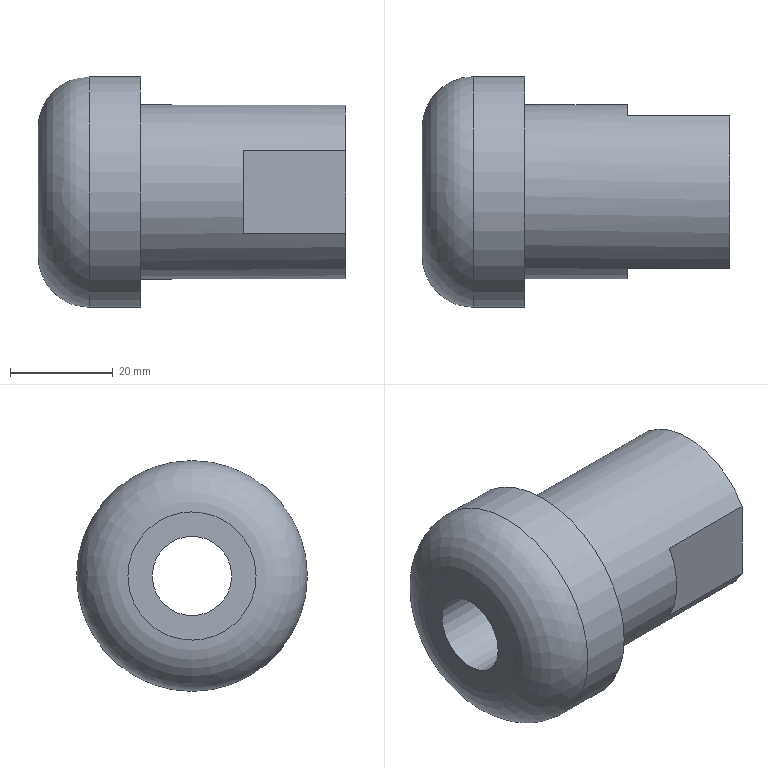Part | NX | features Hydraulic support2 2 | 1 solid | 11 faces | box 60 x 45 x 45 mm | volume 53203 mm3 | plane 7 | cylinder 3 | spline 1 | commonest cylinder face diameters 15.5 x1 34 x1 45 x1